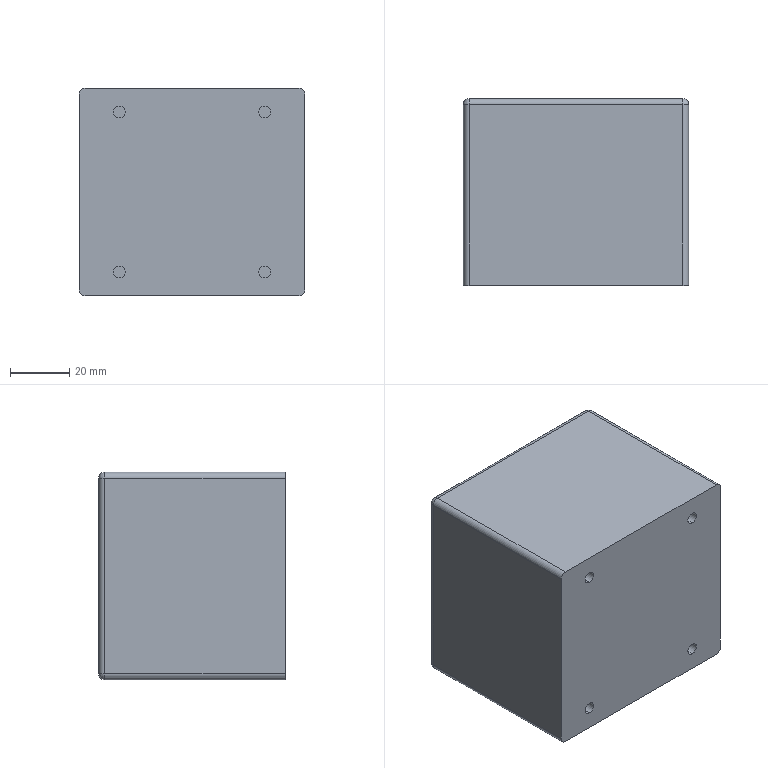Part | STEP file | Button box | 1 solid | 33 faces | box 76 x 63 x 70 mm | volume 332546 mm3 | cylinder 18 | plane 11 | sphere 4 | commonest cylinder face diameters 4 x16 22 x2
STEP:
#1=CARTESIAN_POINT('',(0.,58.,-11.));
#2=VERTEX_POINT('',#1);
#3=CARTESIAN_POINT('',(0.,58.,11.));
#4=VERTEX_POINT('',#3);
#5=CARTESIAN_POINT('',(0.,58.,0.));
#6=DIRECTION('',(0.,1.,0.));
#7=DIRECTION('',(0.,0.,1.));
#8=AXIS2_PLACEMENT_3D('',#5,#6,#7);
#9=CIRCLE('',#8,11.);
#10=EDGE_CURVE('',#2,#4,#9,.T.);
#11=ORIENTED_EDGE('',*,*,#10,.F.);
#12=CARTESIAN_POINT('',(0.,63.,-11.));
#13=VERTEX_POINT('',#12);
#14=CARTESIAN_POINT('',(0.,58.,-11.));
#15=DIRECTION('',(0.,1.,0.));
#16=VECTOR('',#15,1000.);
#17=LINE('',#14,#16);
#18=EDGE_CURVE('',#2,#13,#17,.T.);
#19=ORIENTED_EDGE('',*,*,#18,.T.);
#20=CARTESIAN_POINT('',(0.,63.,11.));
#21=VERTEX_POINT('',#20);
#22=CARTESIAN_POINT('',(0.,63.,0.));
#23=DIRECTION('',(0.,1.,0.));
#24=DIRECTION('',(0.,0.,1.));
#25=AXIS2_PLACEMENT_3D('',#22,#23,#24);
#26=CIRCLE('',#25,11.);
#27=EDGE_CURVE('',#13,#21,#26,.T.);
#28=ORIENTED_EDGE('',*,*,#27,.T.);
#29=CARTESIAN_POINT('',(0.,58.,11.));
#30=DIRECTION('',(0.,1.,0.));
#31=VECTOR('',#30,1000.);
#32=LINE('',#29,#31);
#33=EDGE_CURVE('',#4,#21,#32,.T.);
#34=ORIENTED_EDGE('',*,*,#33,.F.);
#35=EDGE_LOOP('',(#11,#19,#28,#34));
#36=FACE_OUTER_BOUND('',#35,.T.);
#37=CARTESIAN_POINT('',(0.,58.,0.));
#38=DIRECTION('',(0.,1.,0.));
#39=DIRECTION('',(0.,0.,1.));
#40=AXIS2_PLACEMENT_3D('',#37,#38,#39);
#41=CYLINDRICAL_SURFACE('',#40,11.);
#42=ADVANCED_FACE('',(#36),#41,.F.);
#43=CARTESIAN_POINT('',(-24.5,5.,-25.));
#44=VERTEX_POINT('',#43);
#45=CARTESIAN_POINT('',(-24.5,5.,-29.));
#46=VERTEX_POINT('',#45);
#47=CARTESIAN_POINT('',(-24.5,5.,-27.));
#48=DIRECTION('',(0.,-1.,0.));
#49=DIRECTION('',(0.,0.,1.));
#50=AXIS2_PLACEMENT_3D('',#47,#48,#49);
#51=CIRCLE('',#50,2.);
#52=EDGE_CURVE('',#44,#46,#51,.T.);
#53=ORIENTED_EDGE('',*,*,#52,.F.);
#54=CARTESIAN_POINT('',(-24.5,0.,-25.));
#55=VERTEX_POINT('',#54);
#56=CARTESIAN_POINT('',(-24.5,5.,-25.));
#57=DIRECTION('',(0.,-1.,0.));
#58=VECTOR('',#57,1000.);
#59=LINE('',#56,#58);
#60=EDGE_CURVE('',#44,#55,#59,.T.);
#61=ORIENTED_EDGE('',*,*,#60,.T.);
#62=CARTESIAN_POINT('',(-24.5,0.,-29.));
#63=VERTEX_POINT('',#62);
#64=CARTESIAN_POINT('',(-24.5,0.,-27.));
#65=DIRECTION('',(0.,-1.,0.));
#66=DIRECTION('',(0.,0.,1.));
#67=AXIS2_PLACEMENT_3D('',#64,#65,#66);
#68=CIRCLE('',#67,2.);
#69=EDGE_CURVE('',#55,#63,#68,.T.);
#70=ORIENTED_EDGE('',*,*,#69,.T.);
#71=CARTESIAN_POINT('',(-24.5,5.,-29.));
#72=DIRECTION('',(0.,-1.,0.));
#73=VECTOR('',#72,1000.);
#74=LINE('',#71,#73);
#75=EDGE_CURVE('',#46,#63,#74,.T.);
#76=ORIENTED_EDGE('',*,*,#75,.F.);
#77=EDGE_LOOP('',(#53,#61,#70,#76));
#78=FACE_OUTER_BOUND('',#77,.T.);
#79=CARTESIAN_POINT('',(-24.5,5.,-27.));
#80=DIRECTION('',(0.,-1.,0.));
#81=DIRECTION('',(0.,0.,-1.));
#82=AXIS2_PLACEMENT_3D('',#79,#80,#81);
#83=CYLINDRICAL_SURFACE('',#82,2.);
#84=ADVANCED_FACE('',(#78),#83,.F.);
#85=CARTESIAN_POINT('',(24.5,5.,-25.));
#86=VERTEX_POINT('',#85);
#87=CARTESIAN_POINT('',(24.5,5.,-29.));
#88=VERTEX_POINT('',#87);
#89=CARTESIAN_POINT('',(24.5,5.,-27.));
#90=DIRECTION('',(0.,-1.,0.));
#91=DIRECTION('',(0.,0.,-1.));
#92=AXIS2_PLACEMENT_3D('',#89,#90,#91);
#93=CIRCLE('',#92,2.);
#94=EDGE_CURVE('',#86,#88,#93,.T.);
#95=ORIENTED_EDGE('',*,*,#94,.F.);
#96=CARTESIAN_POINT('',(24.5,0.,-25.));
#97=VERTEX_POINT('',#96);
#98=CARTESIAN_POINT('',(24.5,5.,-25.));
#99=DIRECTION('',(0.,-1.,0.));
#100=VECTOR('',#99,1000.);
#101=LINE('',#98,#100);
#102=EDGE_CURVE('',#86,#97,#101,.T.);
#103=ORIENTED_EDGE('',*,*,#102,.T.);
#104=CARTESIAN_POINT('',(24.5,0.,-29.));
#105=VERTEX_POINT('',#104);
#106=CARTESIAN_POINT('',(24.5,0.,-27.));
#107=DIRECTION('',(0.,-1.,0.));
#108=DIRECTION('',(0.,0.,-1.));
#109=AXIS2_PLACEMENT_3D('',#106,#107,#108);
#110=CIRCLE('',#109,2.);
#111=EDGE_CURVE('',#97,#105,#110,.T.);
#112=ORIENTED_EDGE('',*,*,#111,.T.);
#113=CARTESIAN_POINT('',(24.5,5.,-29.));
#114=DIRECTION('',(0.,-1.,0.));
#115=VECTOR('',#114,1000.);
#116=LINE('',#113,#115);
#117=EDGE_CURVE('',#88,#105,#116,.T.);
#118=ORIENTED_EDGE('',*,*,#117,.F.);
#119=EDGE_LOOP('',(#95,#103,#112,#118));
#120=FACE_OUTER_BOUND('',#119,.T.);
#121=CARTESIAN_POINT('',(24.5,5.,-27.));
#122=DIRECTION('',(0.,-1.,0.));
#123=DIRECTION('',(0.,0.,-1.));
#124=AXIS2_PLACEMENT_3D('',#121,#122,#123);
#125=CYLINDRICAL_SURFACE('',#124,2.);
#126=ADVANCED_FACE('',(#120),#125,.F.);
#127=CARTESIAN_POINT('',(24.5,5.,29.));
#128=VERTEX_POINT('',#127);
#129=CARTESIAN_POINT('',(24.5,5.,25.));
#130=VERTEX_POINT('',#129);
#131=CARTESIAN_POINT('',(24.5,5.,27.));
#132=DIRECTION('',(0.,-1.,0.));
#133=DIRECTION('',(0.,0.,1.));
#134=AXIS2_PLACEMENT_3D('',#131,#132,#133);
#135=CIRCLE('',#134,2.);
#136=EDGE_CURVE('',#128,#130,#135,.T.);
#137=ORIENTED_EDGE('',*,*,#136,.F.);
#138=CARTESIAN_POINT('',(24.5,0.,29.));
#139=VERTEX_POINT('',#138);
#140=CARTESIAN_POINT('',(24.5,5.,29.));
#141=DIRECTION('',(0.,-1.,0.));
#142=VECTOR('',#141,1000.);
#143=LINE('',#140,#142);
#144=EDGE_CURVE('',#128,#139,#143,.T.);
#145=ORIENTED_EDGE('',*,*,#144,.T.);
#146=CARTESIAN_POINT('',(24.5,0.,25.));
#147=VERTEX_POINT('',#146);
#148=CARTESIAN_POINT('',(24.5,0.,27.));
#149=DIRECTION('',(0.,-1.,0.));
#150=DIRECTION('',(0.,0.,1.));
#151=AXIS2_PLACEMENT_3D('',#148,#149,#150);
#152=CIRCLE('',#151,2.);
#153=EDGE_CURVE('',#139,#147,#152,.T.);
#154=ORIENTED_EDGE('',*,*,#153,.T.);
#155=CARTESIAN_POINT('',(24.5,5.,25.));
#156=DIRECTION('',(0.,-1.,0.));
#157=VECTOR('',#156,1000.);
#158=LINE('',#155,#157);
#159=EDGE_CURVE('',#130,#147,#158,.T.);
#160=ORIENTED_EDGE('',*,*,#159,.F.);
#161=EDGE_LOOP('',(#137,#145,#154,#160));
#162=FACE_OUTER_BOUND('',#161,.T.);
#163=CARTESIAN_POINT('',(24.5,5.,27.));
#164=DIRECTION('',(0.,-1.,0.));
#165=DIRECTION('',(0.,0.,-1.));
#166=AXIS2_PLACEMENT_3D('',#163,#164,#165);
#167=CYLINDRICAL_SURFACE('',#166,2.);
#168=ADVANCED_FACE('',(#162),#167,.F.);
#169=CARTESIAN_POINT('',(-24.5,5.,29.));
#170=VERTEX_POINT('',#169);
#171=CARTESIAN_POINT('',(-24.5,5.,25.));
#172=VERTEX_POINT('',#171);
#173=CARTESIAN_POINT('',(-24.5,5.,27.));
#174=DIRECTION('',(0.,-1.,0.));
#175=DIRECTION('',(0.,0.,-1.));
#176=AXIS2_PLACEMENT_3D('',#173,#174,#175);
#177=CIRCLE('',#176,2.);
#178=EDGE_CURVE('',#170,#172,#177,.T.);
#179=ORIENTED_EDGE('',*,*,#178,.F.);
#180=CARTESIAN_POINT('',(-24.5,0.,29.));
#181=VERTEX_POINT('',#180);
#182=CARTESIAN_POINT('',(-24.5,5.,29.));
#183=DIRECTION('',(0.,-1.,0.));
#184=VECTOR('',#183,1000.);
#185=LINE('',#182,#184);
#186=EDGE_CURVE('',#170,#181,#185,.T.);
#187=ORIENTED_EDGE('',*,*,#186,.T.);
#188=CARTESIAN_POINT('',(-24.5,0.,25.));
#189=VERTEX_POINT('',#188);
#190=CARTESIAN_POINT('',(-24.5,0.,27.));
#191=DIRECTION('',(0.,-1.,0.));
#192=DIRECTION('',(0.,0.,-1.));
#193=AXIS2_PLACEMENT_3D('',#190,#191,#192);
#194=CIRCLE('',#193,2.);
#195=EDGE_CURVE('',#181,#189,#194,.T.);
#196=ORIENTED_EDGE('',*,*,#195,.T.);
#197=CARTESIAN_POINT('',(-24.5,5.,25.));
#198=DIRECTION('',(0.,-1.,0.));
#199=VECTOR('',#198,1000.);
#200=LINE('',#197,#199);
#201=EDGE_CURVE('',#172,#189,#200,.T.);
#202=ORIENTED_EDGE('',*,*,#201,.F.);
#203=EDGE_LOOP('',(#179,#187,#196,#202));
#204=FACE_OUTER_BOUND('',#203,.T.);
#205=CARTESIAN_POINT('',(-24.5,5.,27.));
#206=DIRECTION('',(0.,-1.,0.));
#207=DIRECTION('',(0.,0.,-1.));
#208=AXIS2_PLACEMENT_3D('',#205,#206,#207);
#209=CYLINDRICAL_SURFACE('',#208,2.);
#210=ADVANCED_FACE('',(#204),#209,.F.);
#211=CARTESIAN_POINT('',(38.,61.,-33.));
#212=VERTEX_POINT('',#211);
#213=CARTESIAN_POINT('',(38.,61.,33.));
#214=VERTEX_POINT('',#213);
#215=CARTESIAN_POINT('',(38.,61.,35.));
#216=DIRECTION('',(0.,0.,1.));
#217=VECTOR('',#216,1000.);
#218=LINE('',#215,#217);
#219=EDGE_CURVE('',#212,#214,#218,.T.);
#220=ORIENTED_EDGE('',*,*,#219,.T.);
#221=CARTESIAN_POINT('',(38.,0.,33.));
#222=VERTEX_POINT('',#221);
#223=CARTESIAN_POINT('',(38.,63.,33.));
#224=DIRECTION('',(0.,-1.,0.));
#225=VECTOR('',#224,1000.);
#226=LINE('',#223,#225);
#227=EDGE_CURVE('',#214,#222,#226,.T.);
#228=ORIENTED_EDGE('',*,*,#227,.T.);
#229=CARTESIAN_POINT('',(38.,0.,-33.));
#230=VERTEX_POINT('',#229);
#231=CARTESIAN_POINT('',(38.,0.,-35.));
#232=DIRECTION('',(0.,0.,-1.));
#233=VECTOR('',#232,1000.);
#234=LINE('',#231,#233);
#235=EDGE_CURVE('',#222,#230,#234,.T.);
#236=ORIENTED_EDGE('',*,*,#235,.T.);
#237=CARTESIAN_POINT('',(38.,63.,-33.));
#238=DIRECTION('',(0.,1.,0.));
#239=VECTOR('',#238,1000.);
#240=LINE('',#237,#239);
#241=EDGE_CURVE('',#230,#212,#240,.T.);
#242=ORIENTED_EDGE('',*,*,#241,.T.);
#243=EDGE_LOOP('',(#220,#228,#236,#242));
#244=FACE_OUTER_BOUND('',#243,.T.);
#245=CARTESIAN_POINT('',(38.,63.,-35.));
#246=DIRECTION('',(-1.,0.,0.));
#247=DIRECTION('',(0.,0.,1.));
#248=AXIS2_PLACEMENT_3D('',#245,#246,#247);
#249=PLANE('',#248);
#250=ADVANCED_FACE('',(#244),#249,.F.);
#251=CARTESIAN_POINT('',(-36.,61.,-35.));
#252=VERTEX_POINT('',#251);
#253=CARTESIAN_POINT('',(36.,61.,-35.));
#254=VERTEX_POINT('',#253);
#255=CARTESIAN_POINT('',(38.,61.,-35.));
#256=DIRECTION('',(1.,0.,0.));
#257=VECTOR('',#256,1000.);
#258=LINE('',#255,#257);
#259=EDGE_CURVE('',#252,#254,#258,.T.);
#260=ORIENTED_EDGE('',*,*,#259,.T.);
#261=CARTESIAN_POINT('',(36.,0.,-35.));
#262=VERTEX_POINT('',#261);
#263=CARTESIAN_POINT('',(36.,63.,-35.));
#264=DIRECTION('',(0.,-1.,0.));
#265=VECTOR('',#264,1000.);
#266=LINE('',#263,#265);
#267=EDGE_CURVE('',#254,#262,#266,.T.);
#268=ORIENTED_EDGE('',*,*,#267,.T.);
#269=CARTESIAN_POINT('',(-36.,0.,-35.));
#270=VERTEX_POINT('',#269);
#271=CARTESIAN_POINT('',(-38.,0.,-35.));
#272=DIRECTION('',(-1.,0.,0.));
#273=VECTOR('',#272,1000.);
#274=LINE('',#271,#273);
#275=EDGE_CURVE('',#262,#270,#274,.T.);
#276=ORIENTED_EDGE('',*,*,#275,.T.);
#277=CARTESIAN_POINT('',(-36.,63.,-35.));
#278=DIRECTION('',(0.,1.,0.));
#279=VECTOR('',#278,1000.);
#280=LINE('',#277,#279);
#281=EDGE_CURVE('',#270,#252,#280,.T.);
#282=ORIENTED_EDGE('',*,*,#281,.T.);
#283=EDGE_LOOP('',(#260,#268,#276,#282));
#284=FACE_OUTER_BOUND('',#283,.T.);
#285=CARTESIAN_POINT('',(-38.,63.,-35.));
#286=DIRECTION('',(0.,0.,1.));
#287=DIRECTION('',(1.,0.,0.));
#288=AXIS2_PLACEMENT_3D('',#285,#286,#287);
#289=PLANE('',#288);
#290=ADVANCED_FACE('',(#284),#289,.F.);
#291=CARTESIAN_POINT('',(-38.,0.,-33.));
#292=VERTEX_POINT('',#291);
#293=CARTESIAN_POINT('',(-38.,0.,33.));
#294=VERTEX_POINT('',#293);
#295=CARTESIAN_POINT('',(-38.,0.,-35.));
#296=DIRECTION('',(0.,0.,1.));
#297=VECTOR('',#296,1000.);
#298=LINE('',#295,#297);
#299=EDGE_CURVE('',#292,#294,#298,.T.);
#300=ORIENTED_EDGE('',*,*,#299,.T.);
#301=CARTESIAN_POINT('',(-38.,61.,33.));
#302=VERTEX_POINT('',#301);
#303=CARTESIAN_POINT('',(-38.,63.,33.));
#304=DIRECTION('',(0.,1.,0.));
#305=VECTOR('',#304,1000.);
#306=LINE('',#303,#305);
#307=EDGE_CURVE('',#294,#302,#306,.T.);
#308=ORIENTED_EDGE('',*,*,#307,.T.);
#309=CARTESIAN_POINT('',(-38.,61.,-33.));
#310=VERTEX_POINT('',#309);
#311=CARTESIAN_POINT('',(-38.,61.,-35.));
#312=DIRECTION('',(0.,0.,-1.));
#313=VECTOR('',#312,1000.);
#314=LINE('',#311,#313);
#315=EDGE_CURVE('',#302,#310,#314,.T.);
#316=ORIENTED_EDGE('',*,*,#315,.T.);
#317=CARTESIAN_POINT('',(-38.,63.,-33.));
#318=DIRECTION('',(0.,-1.,0.));
#319=VECTOR('',#318,1000.);
#320=LINE('',#317,#319);
#321=EDGE_CURVE('',#310,#292,#320,.T.);
#322=ORIENTED_EDGE('',*,*,#321,.T.);
#323=EDGE_LOOP('',(#300,#308,#316,#322));
#324=FACE_OUTER_BOUND('',#323,.T.);
#325=CARTESIAN_POINT('',(-38.,63.,-35.));
#326=DIRECTION('',(1.,0.,0.));
#327=DIRECTION('',(0.,0.,-1.));
#328=AXIS2_PLACEMENT_3D('',#325,#326,#327);
#329=PLANE('',#328);
#330=ADVANCED_FACE('',(#324),#329,.F.);
#331=CARTESIAN_POINT('',(-36.,0.,35.));
#332=VERTEX_POINT('',#331);
#333=CARTESIAN_POINT('',(36.,0.,35.));
#334=VERTEX_POINT('',#333);
#335=CARTESIAN_POINT('',(-38.,0.,35.));
#336=DIRECTION('',(1.,0.,0.));
#337=VECTOR('',#336,1000.);
#338=LINE('',#335,#337);
#339=EDGE_CURVE('',#332,#334,#338,.T.);
#340=ORIENTED_EDGE('',*,*,#339,.T.);
#341=CARTESIAN_POINT('',(36.,61.,35.));
#342=VERTEX_POINT('',#341);
#343=CARTESIAN_POINT('',(36.,63.,35.));
#344=DIRECTION('',(0.,1.,0.));
#345=VECTOR('',#344,1000.);
#346=LINE('',#343,#345);
#347=EDGE_CURVE('',#334,#342,#346,.T.);
#348=ORIENTED_EDGE('',*,*,#347,.T.);
#349=CARTESIAN_POINT('',(-36.,61.,35.));
#350=VERTEX_POINT('',#349);
#351=CARTESIAN_POINT('',(-38.,61.,35.));
#352=DIRECTION('',(-1.,0.,0.));
#353=VECTOR('',#352,1000.);
#354=LINE('',#351,#353);
#355=EDGE_CURVE('',#342,#350,#354,.T.);
#356=ORIENTED_EDGE('',*,*,#355,.T.);
#357=CARTESIAN_POINT('',(-36.,63.,35.));
#358=DIRECTION('',(0.,-1.,0.));
#359=VECTOR('',#358,1000.);
#360=LINE('',#357,#359);
#361=EDGE_CURVE('',#350,#332,#360,.T.);
#362=ORIENTED_EDGE('',*,*,#361,.T.);
#363=EDGE_LOOP('',(#340,#348,#356,#362));
#364=FACE_OUTER_BOUND('',#363,.T.);
#365=CARTESIAN_POINT('',(-38.,63.,35.));
#366=DIRECTION('',(0.,0.,-1.));
#367=DIRECTION('',(-1.,0.,0.));
#368=AXIS2_PLACEMENT_3D('',#365,#366,#367);
#369=PLANE('',#368);
#370=ADVANCED_FACE('',(#364),#369,.F.);
#371=CARTESIAN_POINT('',(0.,63.,0.));
#372=DIRECTION('',(0.,1.,0.));
#373=DIRECTION('',(0.,0.,1.));
#374=AXIS2_PLACEMENT_3D('',#371,#372,#373);
#375=CIRCLE('',#374,11.);
#376=EDGE_CURVE('',#21,#13,#375,.T.);
#377=ORIENTED_EDGE('',*,*,#376,.F.);
#378=ORIENTED_EDGE('',*,*,#27,.F.);
#379=EDGE_LOOP('',(#377,#378));
#380=FACE_BOUND('',#379,.T.);
#381=CARTESIAN_POINT('',(-36.,63.,-33.));
#382=VERTEX_POINT('',#381);
#383=CARTESIAN_POINT('',(-36.,63.,33.));
#384=VERTEX_POINT('',#383);
#385=CARTESIAN_POINT('',(-36.,63.,35.));
#386=DIRECTION('',(0.,0.,1.));
#387=VECTOR('',#386,1000.);
#388=LINE('',#385,#387);
#389=EDGE_CURVE('',#382,#384,#388,.T.);
#390=ORIENTED_EDGE('',*,*,#389,.T.);
#391=CARTESIAN_POINT('',(36.,63.,33.));
#392=VERTEX_POINT('',#391);
#393=CARTESIAN_POINT('',(38.,63.,33.));
#394=DIRECTION('',(1.,0.,0.));
#395=VECTOR('',#394,1000.);
#396=LINE('',#393,#395);
#397=EDGE_CURVE('',#384,#392,#396,.T.);
#398=ORIENTED_EDGE('',*,*,#397,.T.);
#399=CARTESIAN_POINT('',(36.,63.,-33.));
#400=VERTEX_POINT('',#399);
#401=CARTESIAN_POINT('',(36.,63.,-35.));
#402=DIRECTION('',(0.,0.,-1.));
#403=VECTOR('',#402,1000.);
#404=LINE('',#401,#403);
#405=EDGE_CURVE('',#392,#400,#404,.T.);
#406=ORIENTED_EDGE('',*,*,#405,.T.);
#407=CARTESIAN_POINT('',(-38.,63.,-33.));
#408=DIRECTION('',(-1.,0.,0.));
#409=VECTOR('',#408,1000.);
#410=LINE('',#407,#409);
#411=EDGE_CURVE('',#400,#382,#410,.T.);
#412=ORIENTED_EDGE('',*,*,#411,.T.);
#413=EDGE_LOOP('',(#390,#398,#406,#412));
#414=FACE_OUTER_BOUND('',#413,.T.);
#415=CARTESIAN_POINT('',(38.,63.,35.));
#416=DIRECTION('',(0.,1.,0.));
#417=DIRECTION('',(0.,0.,1.));
#418=AXIS2_PLACEMENT_3D('',#415,#416,#417);
#419=PLANE('',#418);
#420=ADVANCED_FACE('',(#380,#414),#419,.T.);
#421=CARTESIAN_POINT('',(-24.5,0.,-27.));
#422=DIRECTION('',(0.,-1.,0.));
#423=DIRECTION('',(0.,0.,1.));
#424=AXIS2_PLACEMENT_3D('',#421,#422,#423);
#425=CIRCLE('',#424,2.);
#426=EDGE_CURVE('',#63,#55,#425,.T.);
#427=ORIENTED_EDGE('',*,*,#426,.F.);
#428=ORIENTED_EDGE('',*,*,#69,.F.);
#429=EDGE_LOOP('',(#427,#428));
#430=FACE_BOUND('',#429,.T.);
#431=CARTESIAN_POINT('',(24.5,0.,-27.));
#432=DIRECTION('',(0.,-1.,0.));
#433=DIRECTION('',(0.,0.,-1.));
#434=AXIS2_PLACEMENT_3D('',#431,#432,#433);
#435=CIRCLE('',#434,2.);
#436=EDGE_CURVE('',#105,#97,#435,.T.);
#437=ORIENTED_EDGE('',*,*,#436,.F.);
#438=ORIENTED_EDGE('',*,*,#111,.F.);
#439=EDGE_LOOP('',(#437,#438));
#440=FACE_BOUND('',#439,.T.);
#441=CARTESIAN_POINT('',(24.5,0.,27.));
#442=DIRECTION('',(0.,-1.,0.));
#443=DIRECTION('',(0.,0.,1.));
#444=AXIS2_PLACEMENT_3D('',#441,#442,#443);
#445=CIRCLE('',#444,2.);
#446=EDGE_CURVE('',#147,#139,#445,.T.);
#447=ORIENTED_EDGE('',*,*,#446,.F.);
#448=ORIENTED_EDGE('',*,*,#153,.F.);
#449=EDGE_LOOP('',(#447,#448));
#450=FACE_BOUND('',#449,.T.);
#451=CARTESIAN_POINT('',(-24.5,0.,27.));
#452=DIRECTION('',(0.,-1.,0.));
#453=DIRECTION('',(0.,0.,-1.));
#454=AXIS2_PLACEMENT_3D('',#451,#452,#453);
#455=CIRCLE('',#454,2.);
#456=EDGE_CURVE('',#189,#181,#455,.T.);
#457=ORIENTED_EDGE('',*,*,#456,.F.);
#458=ORIENTED_EDGE('',*,*,#195,.F.);
#459=EDGE_LOOP('',(#457,#458));
#460=FACE_BOUND('',#459,.T.);
#461=ORIENTED_EDGE('',*,*,#235,.F.);
#462=CARTESIAN_POINT('',(36.,0.,33.));
#463=DIRECTION('',(0.,-1.,0.));
#464=DIRECTION('',(0.,0.,1.));
#465=AXIS2_PLACEMENT_3D('',#462,#463,#464);
#466=CIRCLE('',#465,2.);
#467=EDGE_CURVE('',#222,#334,#466,.T.);
#468=ORIENTED_EDGE('',*,*,#467,.T.);
#469=ORIENTED_EDGE('',*,*,#339,.F.);
#470=CARTESIAN_POINT('',(-36.,0.,33.));
#471=DIRECTION('',(0.,-1.,0.));
#472=DIRECTION('',(0.,0.,1.));
#473=AXIS2_PLACEMENT_3D('',#470,#471,#472);
#474=CIRCLE('',#473,2.);
#475=EDGE_CURVE('',#332,#294,#474,.T.);
#476=ORIENTED_EDGE('',*,*,#475,.T.);
#477=ORIENTED_EDGE('',*,*,#299,.F.);
#478=CARTESIAN_POINT('',(-36.,0.,-33.));
#479=DIRECTION('',(0.,-1.,0.));
#480=DIRECTION('',(0.,0.,1.));
#481=AXIS2_PLACEMENT_3D('',#478,#479,#480);
#482=CIRCLE('',#481,2.);
#483=EDGE_CURVE('',#292,#270,#482,.T.);
#484=ORIENTED_EDGE('',*,*,#483,.T.);
#485=ORIENTED_EDGE('',*,*,#275,.F.);
#486=CARTESIAN_POINT('',(36.,0.,-33.));
#487=DIRECTION('',(0.,-1.,0.));
#488=DIRECTION('',(0.,0.,1.));
#489=AXIS2_PLACEMENT_3D('',#486,#487,#488);
#490=CIRCLE('',#489,2.);
#491=EDGE_CURVE('',#262,#230,#490,.T.);
#492=ORIENTED_EDGE('',*,*,#491,.T.);
#493=EDGE_LOOP('',(#461,#468,#469,#476,#477,#484,#485,#492));
#494=FACE_OUTER_BOUND('',#493,.T.);
#495=CARTESIAN_POINT('',(38.,0.,35.));
#496=DIRECTION('',(0.,1.,0.));
#497=DIRECTION('',(0.,0.,1.));
#498=AXIS2_PLACEMENT_3D('',#495,#496,#497);
#499=PLANE('',#498);
#500=ADVANCED_FACE('',(#430,#440,#450,#460,#494),#499,.F.);
#501=ORIENTED_EDGE('',*,*,#483,.F.);
#502=ORIENTED_EDGE('',*,*,#321,.F.);
#503=CARTESIAN_POINT('',(-36.,61.,-33.));
#504=DIRECTION('',(0.,1.,0.));
#505=DIRECTION('',(0.,0.,1.));
#506=AXIS2_PLACEMENT_3D('',#503,#504,#505);
#507=CIRCLE('',#506,2.);
#508=EDGE_CURVE('',#252,#310,#507,.T.);
#509=ORIENTED_EDGE('',*,*,#508,.F.);
#510=ORIENTED_EDGE('',*,*,#281,.F.);
#511=EDGE_LOOP('',(#501,#502,#509,#510));
#512=FACE_OUTER_BOUND('',#511,.T.);
#513=CARTESIAN_POINT('',(-36.,63.,-33.));
#514=DIRECTION('',(0.,-1.,0.));
#515=DIRECTION('',(0.,0.,-1.));
#516=AXIS2_PLACEMENT_3D('',#513,#514,#515);
#517=CYLINDRICAL_SURFACE('',#516,2.);
#518=ADVANCED_FACE('',(#512),#517,.T.);
#519=CARTESIAN_POINT('',(36.,61.,-33.));
#520=DIRECTION('',(1.,0.,0.));
#521=DIRECTION('',(0.,0.,-1.));
#522=AXIS2_PLACEMENT_3D('',#519,#520,#521);
#523=CIRCLE('',#522,2.);
#524=EDGE_CURVE('',#254,#400,#523,.T.);
#525=ORIENTED_EDGE('',*,*,#524,.F.);
#526=ORIENTED_EDGE('',*,*,#259,.F.);
#527=CARTESIAN_POINT('',(-36.,61.,-33.));
#528=DIRECTION('',(-1.,0.,0.));
#529=DIRECTION('',(0.,0.,1.));
#530=AXIS2_PLACEMENT_3D('',#527,#528,#529);
#531=CIRCLE('',#530,2.);
#532=EDGE_CURVE('',#382,#252,#531,.T.);
#533=ORIENTED_EDGE('',*,*,#532,.F.);
#534=ORIENTED_EDGE('',*,*,#411,.F.);
#535=EDGE_LOOP('',(#525,#526,#533,#534));
#536=FACE_OUTER_BOUND('',#535,.T.);
#537=CARTESIAN_POINT('',(38.,61.,-33.));
#538=DIRECTION('',(1.,0.,0.));
#539=DIRECTION('',(0.,0.,-1.));
#540=AXIS2_PLACEMENT_3D('',#537,#538,#539);
#541=CYLINDRICAL_SURFACE('',#540,2.);
#542=ADVANCED_FACE('',(#536),#541,.T.);
#543=ORIENTED_EDGE('',*,*,#491,.F.);
#544=ORIENTED_EDGE('',*,*,#267,.F.);
#545=CARTESIAN_POINT('',(36.,61.,-33.));
#546=DIRECTION('',(0.,1.,0.));
#547=DIRECTION('',(0.,0.,1.));
#548=AXIS2_PLACEMENT_3D('',#545,#546,#547);
#549=CIRCLE('',#548,2.);
#550=EDGE_CURVE('',#212,#254,#549,.T.);
#551=ORIENTED_EDGE('',*,*,#550,.F.);
#552=ORIENTED_EDGE('',*,*,#241,.F.);
#553=EDGE_LOOP('',(#543,#544,#551,#552));
#554=FACE_OUTER_BOUND('',#553,.T.);
#555=CARTESIAN_POINT('',(36.,63.,-33.));
#556=DIRECTION('',(0.,-1.,0.));
#557=DIRECTION('',(0.,0.,-1.));
#558=AXIS2_PLACEMENT_3D('',#555,#556,#557);
#559=CYLINDRICAL_SURFACE('',#558,2.);
#560=ADVANCED_FACE('',(#554),#559,.T.);
#561=ORIENTED_EDGE('',*,*,#532,.T.);
#562=ORIENTED_EDGE('',*,*,#508,.T.);
#563=CARTESIAN_POINT('',(-36.,61.,-33.));
#564=DIRECTION('',(0.,0.,1.));
#565=DIRECTION('',(-1.,0.,0.));
#566=AXIS2_PLACEMENT_3D('',#563,#564,#565);
#567=CIRCLE('',#566,2.);
#568=EDGE_CURVE('',#382,#310,#567,.T.);
#569=ORIENTED_EDGE('',*,*,#568,.F.);
#570=EDGE_LOOP('',(#561,#562,#569));
#571=FACE_OUTER_BOUND('',#570,.T.);
#572=CARTESIAN_POINT('',(-36.,61.,-33.));
#573=DIRECTION('',(0.,1.,0.));
#574=DIRECTION('',(1.,0.,0.));
#575=AXIS2_PLACEMENT_3D('',#572,#573,#574);
#576=SPHERICAL_SURFACE('',#575,2.);
#577=ADVANCED_FACE('',(#571),#576,.T.);
#578=ORIENTED_EDGE('',*,*,#550,.T.);
#579=ORIENTED_EDGE('',*,*,#524,.T.);
#580=CARTESIAN_POINT('',(36.,61.,-33.));
#581=DIRECTION('',(0.,0.,1.));
#582=DIRECTION('',(-1.,0.,0.));
#583=AXIS2_PLACEMENT_3D('',#580,#581,#582);
#584=CIRCLE('',#583,2.);
#585=EDGE_CURVE('',#212,#400,#584,.T.);
#586=ORIENTED_EDGE('',*,*,#585,.F.);
#587=EDGE_LOOP('',(#578,#579,#586));
#588=FACE_OUTER_BOUND('',#587,.T.);
#589=CARTESIAN_POINT('',(36.,61.,-33.));
#590=DIRECTION('',(0.,1.,0.));
#591=DIRECTION('',(1.,0.,0.));
#592=AXIS2_PLACEMENT_3D('',#589,#590,#591);
#593=SPHERICAL_SURFACE('',#592,2.);
#594=ADVANCED_FACE('',(#588),#593,.T.);
#595=ORIENTED_EDGE('',*,*,#475,.F.);
#596=ORIENTED_EDGE('',*,*,#361,.F.);
#597=CARTESIAN_POINT('',(-36.,61.,33.));
#598=DIRECTION('',(0.,1.,0.));
#599=DIRECTION('',(0.,0.,1.));
#600=AXIS2_PLACEMENT_3D('',#597,#598,#599);
#601=CIRCLE('',#600,2.);
#602=EDGE_CURVE('',#302,#350,#601,.T.);
#603=ORIENTED_EDGE('',*,*,#602,.F.);
#604=ORIENTED_EDGE('',*,*,#307,.F.);
#605=EDGE_LOOP('',(#595,#596,#603,#604));
#606=FACE_OUTER_BOUND('',#605,.T.);
#607=CARTESIAN_POINT('',(-36.,63.,33.));
#608=DIRECTION('',(0.,-1.,0.));
#609=DIRECTION('',(0.,0.,-1.));
#610=AXIS2_PLACEMENT_3D('',#607,#608,#609);
#611=CYLINDRICAL_SURFACE('',#610,2.);
#612=ADVANCED_FACE('',(#606),#611,.T.);
#613=ORIENTED_EDGE('',*,*,#568,.T.);
#614=ORIENTED_EDGE('',*,*,#315,.F.);
#615=CARTESIAN_POINT('',(-36.,61.,33.));
#616=DIRECTION('',(0.,0.,1.));
#617=DIRECTION('',(1.,0.,0.));
#618=AXIS2_PLACEMENT_3D('',#615,#616,#617);
#619=CIRCLE('',#618,2.);
#620=EDGE_CURVE('',#384,#302,#619,.T.);
#621=ORIENTED_EDGE('',*,*,#620,.F.);
#622=ORIENTED_EDGE('',*,*,#389,.F.);
#623=EDGE_LOOP('',(#613,#614,#621,#622));
#624=FACE_OUTER_BOUND('',#623,.T.);
#625=CARTESIAN_POINT('',(-36.,61.,35.));
#626=DIRECTION('',(0.,0.,-1.));
#627=DIRECTION('',(-1.,0.,0.));
#628=AXIS2_PLACEMENT_3D('',#625,#626,#627);
#629=CYLINDRICAL_SURFACE('',#628,2.);
#630=ADVANCED_FACE('',(#624),#629,.T.);
#631=ORIENTED_EDGE('',*,*,#585,.T.);
#632=ORIENTED_EDGE('',*,*,#405,.F.);
#633=CARTESIAN_POINT('',(36.,61.,33.));
#634=DIRECTION('',(0.,0.,1.));
#635=DIRECTION('',(1.,0.,0.));
#636=AXIS2_PLACEMENT_3D('',#633,#634,#635);
#637=CIRCLE('',#636,2.);
#638=EDGE_CURVE('',#214,#392,#637,.T.);
#639=ORIENTED_EDGE('',*,*,#638,.F.);
#640=ORIENTED_EDGE('',*,*,#219,.F.);
#641=EDGE_LOOP('',(#631,#632,#639,#640));
#642=FACE_OUTER_BOUND('',#641,.T.);
#643=CARTESIAN_POINT('',(36.,61.,35.));
#644=DIRECTION('',(0.,0.,1.));
#645=DIRECTION('',(1.,0.,0.));
#646=AXIS2_PLACEMENT_3D('',#643,#644,#645);
#647=CYLINDRICAL_SURFACE('',#646,2.);
#648=ADVANCED_FACE('',(#642),#647,.T.);
#649=ORIENTED_EDGE('',*,*,#467,.F.);
#650=ORIENTED_EDGE('',*,*,#227,.F.);
#651=CARTESIAN_POINT('',(36.,61.,33.));
#652=DIRECTION('',(0.,1.,0.));
#653=DIRECTION('',(0.,0.,1.));
#654=AXIS2_PLACEMENT_3D('',#651,#652,#653);
#655=CIRCLE('',#654,2.);
#656=EDGE_CURVE('',#342,#214,#655,.T.);
#657=ORIENTED_EDGE('',*,*,#656,.F.);
#658=ORIENTED_EDGE('',*,*,#347,.F.);
#659=EDGE_LOOP('',(#649,#650,#657,#658));
#660=FACE_OUTER_BOUND('',#659,.T.);
#661=CARTESIAN_POINT('',(36.,63.,33.));
#662=DIRECTION('',(0.,-1.,0.));
#663=DIRECTION('',(0.,0.,-1.));
#664=AXIS2_PLACEMENT_3D('',#661,#662,#663);
#665=CYLINDRICAL_SURFACE('',#664,2.);
#666=ADVANCED_FACE('',(#660),#665,.T.);
#667=ORIENTED_EDGE('',*,*,#620,.T.);
#668=ORIENTED_EDGE('',*,*,#602,.T.);
#669=CARTESIAN_POINT('',(-36.,61.,33.));
#670=DIRECTION('',(1.,0.,0.));
#671=DIRECTION('',(0.,0.,1.));
#672=AXIS2_PLACEMENT_3D('',#669,#670,#671);
#673=CIRCLE('',#672,2.);
#674=EDGE_CURVE('',#384,#350,#673,.T.);
#675=ORIENTED_EDGE('',*,*,#674,.F.);
#676=EDGE_LOOP('',(#667,#668,#675));
#677=FACE_OUTER_BOUND('',#676,.T.);
#678=CARTESIAN_POINT('',(-36.,61.,33.));
#679=DIRECTION('',(0.,1.,0.));
#680=DIRECTION('',(1.,0.,0.));
#681=AXIS2_PLACEMENT_3D('',#678,#679,#680);
#682=SPHERICAL_SURFACE('',#681,2.);
#683=ADVANCED_FACE('',(#677),#682,.T.);
#684=ORIENTED_EDGE('',*,*,#656,.T.);
#685=ORIENTED_EDGE('',*,*,#638,.T.);
#686=CARTESIAN_POINT('',(36.,61.,33.));
#687=DIRECTION('',(-1.,0.,0.));
#688=DIRECTION('',(0.,0.,-1.));
#689=AXIS2_PLACEMENT_3D('',#686,#687,#688);
#690=CIRCLE('',#689,2.);
#691=EDGE_CURVE('',#342,#392,#690,.T.);
#692=ORIENTED_EDGE('',*,*,#691,.F.);
#693=EDGE_LOOP('',(#684,#685,#692));
#694=FACE_OUTER_BOUND('',#693,.T.);
#695=CARTESIAN_POINT('',(36.,61.,33.));
#696=DIRECTION('',(0.,1.,0.));
#697=DIRECTION('',(1.,0.,0.));
#698=AXIS2_PLACEMENT_3D('',#695,#696,#697);
#699=SPHERICAL_SURFACE('',#698,2.);
#700=ADVANCED_FACE('',(#694),#699,.T.);
#701=ORIENTED_EDGE('',*,*,#674,.T.);
#702=ORIENTED_EDGE('',*,*,#355,.F.);
#703=ORIENTED_EDGE('',*,*,#691,.T.);
#704=ORIENTED_EDGE('',*,*,#397,.F.);
#705=EDGE_LOOP('',(#701,#702,#703,#704));
#706=FACE_OUTER_BOUND('',#705,.T.);
#707=CARTESIAN_POINT('',(38.,61.,33.));
#708=DIRECTION('',(-1.,0.,0.));
#709=DIRECTION('',(0.,0.,1.));
#710=AXIS2_PLACEMENT_3D('',#707,#708,#709);
#711=CYLINDRICAL_SURFACE('',#710,2.);
#712=ADVANCED_FACE('',(#706),#711,.T.);
#713=ORIENTED_EDGE('',*,*,#186,.F.);
#714=CARTESIAN_POINT('',(-24.5,5.,27.));
#715=DIRECTION('',(0.,-1.,0.));
#716=DIRECTION('',(0.,0.,-1.));
#717=AXIS2_PLACEMENT_3D('',#714,#715,#716);
#718=CIRCLE('',#717,2.);
#719=EDGE_CURVE('',#172,#170,#718,.T.);
#720=ORIENTED_EDGE('',*,*,#719,.F.);
#721=ORIENTED_EDGE('',*,*,#201,.T.);
#722=ORIENTED_EDGE('',*,*,#456,.T.);
#723=EDGE_LOOP('',(#713,#720,#721,#722));
#724=FACE_OUTER_BOUND('',#723,.T.);
#725=CARTESIAN_POINT('',(-24.5,5.,27.));
#726=DIRECTION('',(0.,-1.,0.));
#727=DIRECTION('',(0.,0.,-1.));
#728=AXIS2_PLACEMENT_3D('',#725,#726,#727);
#729=CYLINDRICAL_SURFACE('',#728,2.);
#730=ADVANCED_FACE('',(#724),#729,.F.);
#731=ORIENTED_EDGE('',*,*,#719,.T.);
#732=ORIENTED_EDGE('',*,*,#178,.T.);
#733=EDGE_LOOP('',(#731,#732));
#734=FACE_OUTER_BOUND('',#733,.T.);
#735=CARTESIAN_POINT('',(-24.5,5.,27.));
#736=DIRECTION('',(0.,-1.,0.));
#737=DIRECTION('',(0.,0.,-1.));
#738=AXIS2_PLACEMENT_3D('',#735,#736,#737);
#739=PLANE('',#738);
#740=ADVANCED_FACE('',(#734),#739,.T.);
#741=ORIENTED_EDGE('',*,*,#144,.F.);
#742=CARTESIAN_POINT('',(24.5,5.,27.));
#743=DIRECTION('',(0.,-1.,0.));
#744=DIRECTION('',(0.,0.,1.));
#745=AXIS2_PLACEMENT_3D('',#742,#743,#744);
#746=CIRCLE('',#745,2.);
#747=EDGE_CURVE('',#130,#128,#746,.T.);
#748=ORIENTED_EDGE('',*,*,#747,.F.);
#749=ORIENTED_EDGE('',*,*,#159,.T.);
#750=ORIENTED_EDGE('',*,*,#446,.T.);
#751=EDGE_LOOP('',(#741,#748,#749,#750));
#752=FACE_OUTER_BOUND('',#751,.T.);
#753=CARTESIAN_POINT('',(24.5,5.,27.));
#754=DIRECTION('',(0.,-1.,0.));
#755=DIRECTION('',(0.,0.,-1.));
#756=AXIS2_PLACEMENT_3D('',#753,#754,#755);
#757=CYLINDRICAL_SURFACE('',#756,2.);
#758=ADVANCED_FACE('',(#752),#757,.F.);
#759=ORIENTED_EDGE('',*,*,#747,.T.);
#760=ORIENTED_EDGE('',*,*,#136,.T.);
#761=EDGE_LOOP('',(#759,#760));
#762=FACE_OUTER_BOUND('',#761,.T.);
#763=CARTESIAN_POINT('',(24.5,5.,27.));
#764=DIRECTION('',(0.,1.,0.));
#765=DIRECTION('',(0.,0.,1.));
#766=AXIS2_PLACEMENT_3D('',#763,#764,#765);
#767=PLANE('',#766);
#768=ADVANCED_FACE('',(#762),#767,.F.);
#769=ORIENTED_EDGE('',*,*,#102,.F.);
#770=CARTESIAN_POINT('',(24.5,5.,-27.));
#771=DIRECTION('',(0.,-1.,0.));
#772=DIRECTION('',(0.,0.,-1.));
#773=AXIS2_PLACEMENT_3D('',#770,#771,#772);
#774=CIRCLE('',#773,2.);
#775=EDGE_CURVE('',#88,#86,#774,.T.);
#776=ORIENTED_EDGE('',*,*,#775,.F.);
#777=ORIENTED_EDGE('',*,*,#117,.T.);
#778=ORIENTED_EDGE('',*,*,#436,.T.);
#779=EDGE_LOOP('',(#769,#776,#777,#778));
#780=FACE_OUTER_BOUND('',#779,.T.);
#781=CARTESIAN_POINT('',(24.5,5.,-27.));
#782=DIRECTION('',(0.,-1.,0.));
#783=DIRECTION('',(0.,0.,-1.));
#784=AXIS2_PLACEMENT_3D('',#781,#782,#783);
#785=CYLINDRICAL_SURFACE('',#784,2.);
#786=ADVANCED_FACE('',(#780),#785,.F.);
#787=ORIENTED_EDGE('',*,*,#775,.T.);
#788=ORIENTED_EDGE('',*,*,#94,.T.);
#789=EDGE_LOOP('',(#787,#788));
#790=FACE_OUTER_BOUND('',#789,.T.);
#791=CARTESIAN_POINT('',(24.5,5.,-27.));
#792=DIRECTION('',(0.,-1.,0.));
#793=DIRECTION('',(0.,0.,-1.));
#794=AXIS2_PLACEMENT_3D('',#791,#792,#793);
#795=PLANE('',#794);
#796=ADVANCED_FACE('',(#790),#795,.T.);
#797=ORIENTED_EDGE('',*,*,#60,.F.);
#798=CARTESIAN_POINT('',(-24.5,5.,-27.));
#799=DIRECTION('',(0.,-1.,0.));
#800=DIRECTION('',(0.,0.,1.));
#801=AXIS2_PLACEMENT_3D('',#798,#799,#800);
#802=CIRCLE('',#801,2.);
#803=EDGE_CURVE('',#46,#44,#802,.T.);
#804=ORIENTED_EDGE('',*,*,#803,.F.);
#805=ORIENTED_EDGE('',*,*,#75,.T.);
#806=ORIENTED_EDGE('',*,*,#426,.T.);
#807=EDGE_LOOP('',(#797,#804,#805,#806));
#808=FACE_OUTER_BOUND('',#807,.T.);
#809=CARTESIAN_POINT('',(-24.5,5.,-27.));
#810=DIRECTION('',(0.,-1.,0.));
#811=DIRECTION('',(0.,0.,-1.));
#812=AXIS2_PLACEMENT_3D('',#809,#810,#811);
#813=CYLINDRICAL_SURFACE('',#812,2.);
#814=ADVANCED_FACE('',(#808),#813,.F.);
#815=ORIENTED_EDGE('',*,*,#803,.T.);
#816=ORIENTED_EDGE('',*,*,#52,.T.);
#817=EDGE_LOOP('',(#815,#816));
#818=FACE_OUTER_BOUND('',#817,.T.);
#819=CARTESIAN_POINT('',(-24.5,5.,-27.));
#820=DIRECTION('',(0.,1.,0.));
#821=DIRECTION('',(0.,0.,1.));
#822=AXIS2_PLACEMENT_3D('',#819,#820,#821);
#823=PLANE('',#822);
#824=ADVANCED_FACE('',(#818),#823,.F.);
#825=ORIENTED_EDGE('',*,*,#18,.F.);
#826=CARTESIAN_POINT('',(0.,58.,0.));
#827=DIRECTION('',(0.,1.,0.));
#828=DIRECTION('',(0.,0.,1.));
#829=AXIS2_PLACEMENT_3D('',#826,#827,#828);
#830=CIRCLE('',#829,11.);
#831=EDGE_CURVE('',#4,#2,#830,.T.);
#832=ORIENTED_EDGE('',*,*,#831,.F.);
#833=ORIENTED_EDGE('',*,*,#33,.T.);
#834=ORIENTED_EDGE('',*,*,#376,.T.);
#835=EDGE_LOOP('',(#825,#832,#833,#834));
#836=FACE_OUTER_BOUND('',#835,.T.);
#837=CARTESIAN_POINT('',(0.,58.,0.));
#838=DIRECTION('',(0.,1.,0.));
#839=DIRECTION('',(0.,0.,1.));
#840=AXIS2_PLACEMENT_3D('',#837,#838,#839);
#841=CYLINDRICAL_SURFACE('',#840,11.);
#842=ADVANCED_FACE('',(#836),#841,.F.);
#843=ORIENTED_EDGE('',*,*,#831,.T.);
#844=ORIENTED_EDGE('',*,*,#10,.T.);
#845=EDGE_LOOP('',(#843,#844));
#846=FACE_OUTER_BOUND('',#845,.T.);
#847=CARTESIAN_POINT('',(0.,58.,0.));
#848=DIRECTION('',(0.,1.,0.));
#849=DIRECTION('',(0.,0.,1.));
#850=AXIS2_PLACEMENT_3D('',#847,#848,#849);
#851=PLANE('',#850);
#852=ADVANCED_FACE('',(#846),#851,.T.);
#853=CLOSED_SHELL('',(#42,#84,#126,#168,#210,#250,#290,#330,#370,#420,#500,#518,#542,#560,#577,#594,#612,#630,#648,#666,#683,#700,#712,#730,#740,#758,#768,#786,#796,#814,#824,#842,#852));
#854=MANIFOLD_SOLID_BREP('',#853);
#855=CARTESIAN_POINT('',(0.,0.,0.));
#856=DIRECTION('',(0.,0.,1.));
#857=DIRECTION('',(1.,0.,0.));
#858=AXIS2_PLACEMENT_3D('',#855,#856,#857);
#859=(LENGTH_UNIT()NAMED_UNIT(*)SI_UNIT(.MILLI.,.METRE.));
#860=UNCERTAINTY_MEASURE_WITH_UNIT(LENGTH_MEASURE(0.00001),#859,'','');
#861=(NAMED_UNIT(*)PLANE_ANGLE_UNIT()SI_UNIT($,.RADIAN.));
#862=(NAMED_UNIT(*)SI_UNIT($,.STERADIAN.)SOLID_ANGLE_UNIT());
#863=(GEOMETRIC_REPRESENTATION_CONTEXT(3)GLOBAL_UNCERTAINTY_ASSIGNED_CONTEXT((#860))GLOBAL_UNIT_ASSIGNED_CONTEXT((#859,#861,#862))REPRESENTATION_CONTEXT('',''));
#864=ADVANCED_BREP_SHAPE_REPRESENTATION('',(#854,#858),#863);